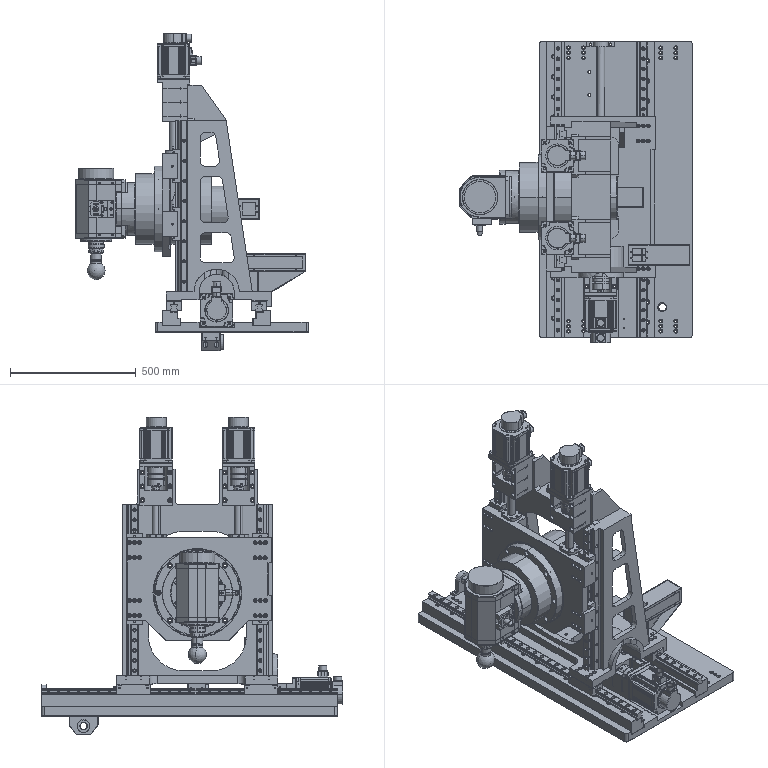Part | SolidWorks | 183 solids | 8559 faces | volume 102091966 mm3 | cylinder 3093 | plane 3004 | cone 1551 | spline 894 | torus 14 | sphere 3 | commonest cylinder face diameters 9 x380 6.5 x340 2 x328 14 x232 5 x190 8.5 x152